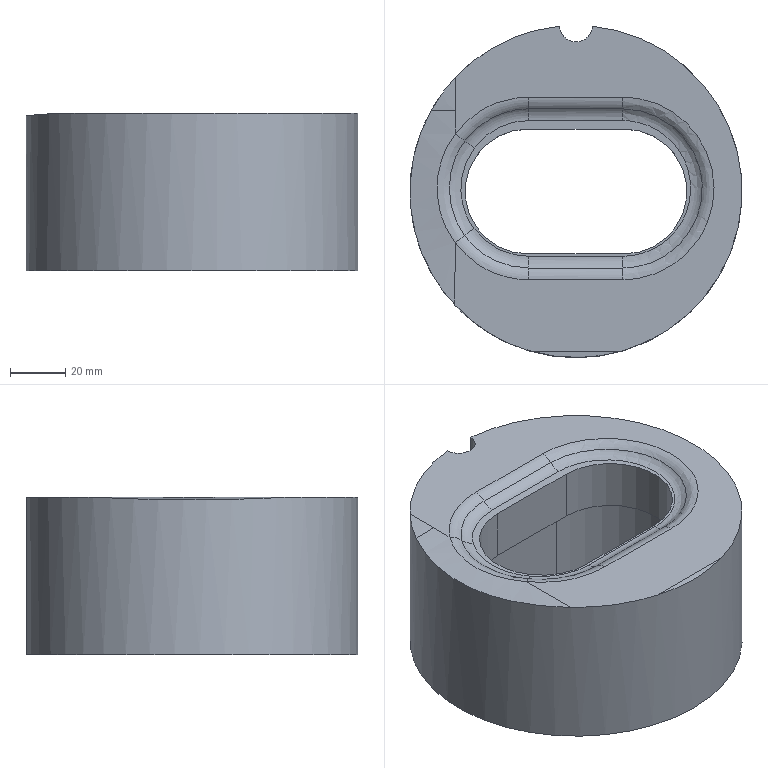Part | NX | features solid 2 | 1 solid | 29 faces | box 120.001 x 119.7 x 57.008 mm | volume 415567 mm3 | cylinder 11 | plane 8 | spline 6 | torus 4 | commonest cylinder face diameters 12 x5 45.1 x2 55.1 x2 20 x1 120 x1